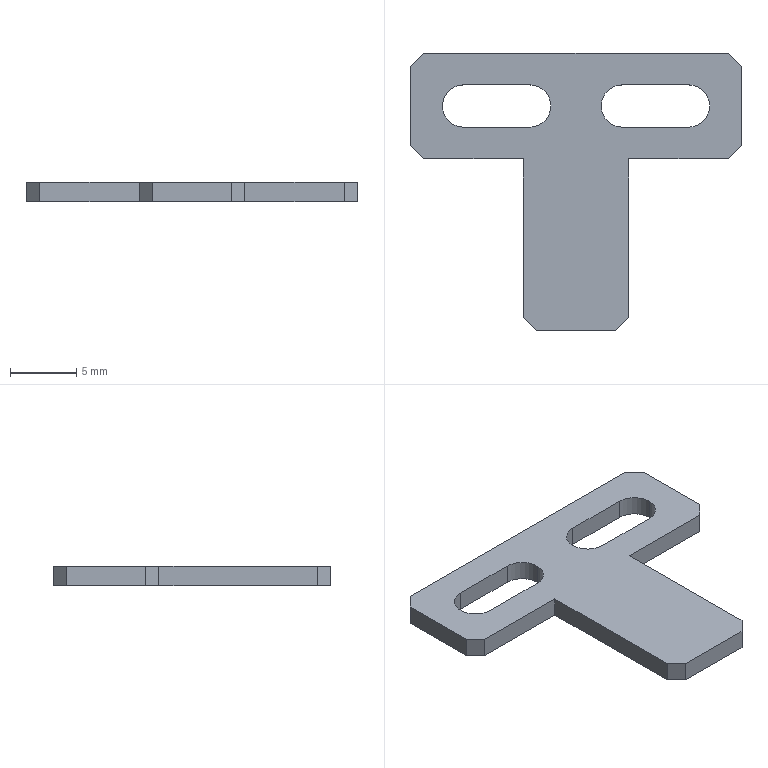Part | SolidWorks | features ICE 2, Chamfer 1, FlatPattern 1, SMBaseFlange 1, SheetMetal 1 | 1 solid | 26 faces | box 25 x 21 x 1.5 mm | volume 379.373 mm3 | plane 20 | cylinder 6 | commonest cylinder face diameters 3.2 x6
STEP:
#1=CARTESIAN_POINT('',(10.1,6.5,-1.5));
#2=VERTEX_POINT('',#1);
#3=CARTESIAN_POINT('',(8.5,8.1,-1.5));
#4=VERTEX_POINT('',#3);
#5=CARTESIAN_POINT('',(8.5,6.5,-1.5));
#6=DIRECTION('',(0.,0.,1.));
#7=DIRECTION('',(1.,0.,0.));
#8=AXIS2_PLACEMENT_3D('',#5,#6,#7);
#9=CIRCLE('',#8,1.6);
#10=EDGE_CURVE('',#2,#4,#9,.T.);
#11=ORIENTED_EDGE('',*,*,#10,.F.);
#12=CARTESIAN_POINT('',(10.1,6.5,0.));
#13=VERTEX_POINT('',#12);
#14=CARTESIAN_POINT('',(10.1,6.5,-1.5));
#15=DIRECTION('',(0.,0.,1.));
#16=VECTOR('',#15,1000.);
#17=LINE('',#14,#16);
#18=EDGE_CURVE('',#2,#13,#17,.T.);
#19=ORIENTED_EDGE('',*,*,#18,.T.);
#20=CARTESIAN_POINT('',(8.5,8.1,0.));
#21=VERTEX_POINT('',#20);
#22=CARTESIAN_POINT('',(8.5,6.5,0.));
#23=DIRECTION('',(0.,0.,1.));
#24=DIRECTION('',(1.,0.,0.));
#25=AXIS2_PLACEMENT_3D('',#22,#23,#24);
#26=CIRCLE('',#25,1.6);
#27=EDGE_CURVE('',#13,#21,#26,.T.);
#28=ORIENTED_EDGE('',*,*,#27,.T.);
#29=CARTESIAN_POINT('',(8.5,8.1,-1.5));
#30=DIRECTION('',(0.,0.,1.));
#31=VECTOR('',#30,1000.);
#32=LINE('',#29,#31);
#33=EDGE_CURVE('',#4,#21,#32,.T.);
#34=ORIENTED_EDGE('',*,*,#33,.F.);
#35=EDGE_LOOP('',(#11,#19,#28,#34));
#36=FACE_OUTER_BOUND('',#35,.T.);
#37=CARTESIAN_POINT('',(8.5,6.5,-1.5));
#38=DIRECTION('',(0.,0.,1.));
#39=DIRECTION('',(1.,0.,0.));
#40=AXIS2_PLACEMENT_3D('',#37,#38,#39);
#41=CYLINDRICAL_SURFACE('',#40,1.6);
#42=ADVANCED_FACE('',(#36),#41,.F.);
#43=CARTESIAN_POINT('',(-1.9,6.5,-1.5));
#44=VERTEX_POINT('',#43);
#45=CARTESIAN_POINT('',(-3.5,8.1,-1.5));
#46=VERTEX_POINT('',#45);
#47=CARTESIAN_POINT('',(-3.5,6.5,-1.5));
#48=DIRECTION('',(0.,0.,1.));
#49=DIRECTION('',(1.,0.,0.));
#50=AXIS2_PLACEMENT_3D('',#47,#48,#49);
#51=CIRCLE('',#50,1.6);
#52=EDGE_CURVE('',#44,#46,#51,.T.);
#53=ORIENTED_EDGE('',*,*,#52,.F.);
#54=CARTESIAN_POINT('',(-1.9,6.5,0.));
#55=VERTEX_POINT('',#54);
#56=CARTESIAN_POINT('',(-1.9,6.5,-1.5));
#57=DIRECTION('',(0.,0.,1.));
#58=VECTOR('',#57,1000.);
#59=LINE('',#56,#58);
#60=EDGE_CURVE('',#44,#55,#59,.T.);
#61=ORIENTED_EDGE('',*,*,#60,.T.);
#62=CARTESIAN_POINT('',(-3.5,8.1,0.));
#63=VERTEX_POINT('',#62);
#64=CARTESIAN_POINT('',(-3.5,6.5,0.));
#65=DIRECTION('',(0.,0.,1.));
#66=DIRECTION('',(1.,0.,0.));
#67=AXIS2_PLACEMENT_3D('',#64,#65,#66);
#68=CIRCLE('',#67,1.6);
#69=EDGE_CURVE('',#55,#63,#68,.T.);
#70=ORIENTED_EDGE('',*,*,#69,.T.);
#71=CARTESIAN_POINT('',(-3.5,8.1,-1.5));
#72=DIRECTION('',(0.,0.,1.));
#73=VECTOR('',#72,1000.);
#74=LINE('',#71,#73);
#75=EDGE_CURVE('',#46,#63,#74,.T.);
#76=ORIENTED_EDGE('',*,*,#75,.F.);
#77=EDGE_LOOP('',(#53,#61,#70,#76));
#78=FACE_OUTER_BOUND('',#77,.T.);
#79=CARTESIAN_POINT('',(-3.5,6.5,-1.5));
#80=DIRECTION('',(0.,0.,1.));
#81=DIRECTION('',(1.,0.,0.));
#82=AXIS2_PLACEMENT_3D('',#79,#80,#81);
#83=CYLINDRICAL_SURFACE('',#82,1.6);
#84=ADVANCED_FACE('',(#78),#83,.F.);
#85=CARTESIAN_POINT('',(12.5,3.5,0.));
#86=VERTEX_POINT('',#85);
#87=CARTESIAN_POINT('',(12.5,9.5,0.));
#88=VERTEX_POINT('',#87);
#89=CARTESIAN_POINT('',(12.5,10.5,0.));
#90=DIRECTION('',(0.,1.,0.));
#91=VECTOR('',#90,1000.);
#92=LINE('',#89,#91);
#93=EDGE_CURVE('',#86,#88,#92,.T.);
#94=ORIENTED_EDGE('',*,*,#93,.F.);
#95=CARTESIAN_POINT('',(12.5,3.5,-1.5));
#96=VERTEX_POINT('',#95);
#97=CARTESIAN_POINT('',(12.5,3.5,-1.5));
#98=DIRECTION('',(0.,0.,-1.));
#99=VECTOR('',#98,1000.);
#100=LINE('',#97,#99);
#101=EDGE_CURVE('',#86,#96,#100,.T.);
#102=ORIENTED_EDGE('',*,*,#101,.T.);
#103=CARTESIAN_POINT('',(12.5,9.5,-1.5));
#104=VERTEX_POINT('',#103);
#105=CARTESIAN_POINT('',(12.5,10.5,-1.5));
#106=DIRECTION('',(0.,1.,0.));
#107=VECTOR('',#106,1000.);
#108=LINE('',#105,#107);
#109=EDGE_CURVE('',#96,#104,#108,.T.);
#110=ORIENTED_EDGE('',*,*,#109,.T.);
#111=CARTESIAN_POINT('',(12.5,9.5,-1.5));
#112=DIRECTION('',(0.,0.,1.));
#113=VECTOR('',#112,1000.);
#114=LINE('',#111,#113);
#115=EDGE_CURVE('',#104,#88,#114,.T.);
#116=ORIENTED_EDGE('',*,*,#115,.T.);
#117=EDGE_LOOP('',(#94,#102,#110,#116));
#118=FACE_OUTER_BOUND('',#117,.T.);
#119=CARTESIAN_POINT('',(12.5,10.5,-1.5));
#120=DIRECTION('',(1.,0.,0.));
#121=DIRECTION('',(0.,1.,0.));
#122=AXIS2_PLACEMENT_3D('',#119,#120,#121);
#123=PLANE('',#122);
#124=ADVANCED_FACE('',(#118),#123,.T.);
#125=CARTESIAN_POINT('',(-3.,-10.5,0.));
#126=VERTEX_POINT('',#125);
#127=CARTESIAN_POINT('',(3.,-10.5,0.));
#128=VERTEX_POINT('',#127);
#129=CARTESIAN_POINT('',(-12.5,-10.5,0.));
#130=DIRECTION('',(1.,0.,0.));
#131=VECTOR('',#130,1000.);
#132=LINE('',#129,#131);
#133=EDGE_CURVE('',#126,#128,#132,.T.);
#134=ORIENTED_EDGE('',*,*,#133,.F.);
#135=CARTESIAN_POINT('',(-3.,-10.5,-1.5));
#136=VERTEX_POINT('',#135);
#137=CARTESIAN_POINT('',(-3.,-10.5,-1.5));
#138=DIRECTION('',(0.,0.,-1.));
#139=VECTOR('',#138,1000.);
#140=LINE('',#137,#139);
#141=EDGE_CURVE('',#126,#136,#140,.T.);
#142=ORIENTED_EDGE('',*,*,#141,.T.);
#143=CARTESIAN_POINT('',(3.,-10.5,-1.5));
#144=VERTEX_POINT('',#143);
#145=CARTESIAN_POINT('',(-12.5,-10.5,-1.5));
#146=DIRECTION('',(1.,0.,0.));
#147=VECTOR('',#146,1000.);
#148=LINE('',#145,#147);
#149=EDGE_CURVE('',#136,#144,#148,.T.);
#150=ORIENTED_EDGE('',*,*,#149,.T.);
#151=CARTESIAN_POINT('',(3.,-10.5,0.));
#152=DIRECTION('',(0.,0.,1.));
#153=VECTOR('',#152,1000.);
#154=LINE('',#151,#153);
#155=EDGE_CURVE('',#144,#128,#154,.T.);
#156=ORIENTED_EDGE('',*,*,#155,.T.);
#157=EDGE_LOOP('',(#134,#142,#150,#156));
#158=FACE_OUTER_BOUND('',#157,.T.);
#159=CARTESIAN_POINT('',(-12.5,-10.5,-1.5));
#160=DIRECTION('',(0.,-1.,0.));
#161=DIRECTION('',(0.,0.,-1.));
#162=AXIS2_PLACEMENT_3D('',#159,#160,#161);
#163=PLANE('',#162);
#164=ADVANCED_FACE('',(#158),#163,.T.);
#165=CARTESIAN_POINT('',(-12.5,9.5,-1.5));
#166=VERTEX_POINT('',#165);
#167=CARTESIAN_POINT('',(-12.5,3.5,-1.5));
#168=VERTEX_POINT('',#167);
#169=CARTESIAN_POINT('',(-12.5,10.5,-1.5));
#170=DIRECTION('',(0.,-1.,0.));
#171=VECTOR('',#170,1000.);
#172=LINE('',#169,#171);
#173=EDGE_CURVE('',#166,#168,#172,.T.);
#174=ORIENTED_EDGE('',*,*,#173,.T.);
#175=CARTESIAN_POINT('',(-12.5,3.5,0.));
#176=VERTEX_POINT('',#175);
#177=CARTESIAN_POINT('',(-12.5,3.5,0.));
#178=DIRECTION('',(0.,0.,1.));
#179=VECTOR('',#178,1000.);
#180=LINE('',#177,#179);
#181=EDGE_CURVE('',#168,#176,#180,.T.);
#182=ORIENTED_EDGE('',*,*,#181,.T.);
#183=CARTESIAN_POINT('',(-12.5,9.5,0.));
#184=VERTEX_POINT('',#183);
#185=CARTESIAN_POINT('',(-12.5,10.5,0.));
#186=DIRECTION('',(0.,-1.,0.));
#187=VECTOR('',#186,1000.);
#188=LINE('',#185,#187);
#189=EDGE_CURVE('',#184,#176,#188,.T.);
#190=ORIENTED_EDGE('',*,*,#189,.F.);
#191=CARTESIAN_POINT('',(-12.5,9.5,-1.5));
#192=DIRECTION('',(0.,0.,-1.));
#193=VECTOR('',#192,1000.);
#194=LINE('',#191,#193);
#195=EDGE_CURVE('',#184,#166,#194,.T.);
#196=ORIENTED_EDGE('',*,*,#195,.T.);
#197=EDGE_LOOP('',(#174,#182,#190,#196));
#198=FACE_OUTER_BOUND('',#197,.T.);
#199=CARTESIAN_POINT('',(-12.5,10.5,-1.5));
#200=DIRECTION('',(-1.,0.,0.));
#201=DIRECTION('',(0.,-1.,0.));
#202=AXIS2_PLACEMENT_3D('',#199,#200,#201);
#203=PLANE('',#202);
#204=ADVANCED_FACE('',(#198),#203,.T.);
#205=CARTESIAN_POINT('',(11.5,10.5,-1.5));
#206=VERTEX_POINT('',#205);
#207=CARTESIAN_POINT('',(-11.5,10.5,-1.5));
#208=VERTEX_POINT('',#207);
#209=CARTESIAN_POINT('',(-12.5,10.5,-1.5));
#210=DIRECTION('',(-1.,0.,0.));
#211=VECTOR('',#210,1000.);
#212=LINE('',#209,#211);
#213=EDGE_CURVE('',#206,#208,#212,.T.);
#214=ORIENTED_EDGE('',*,*,#213,.T.);
#215=CARTESIAN_POINT('',(-11.5,10.5,0.));
#216=VERTEX_POINT('',#215);
#217=CARTESIAN_POINT('',(-11.5,10.5,-1.5));
#218=DIRECTION('',(0.,0.,1.));
#219=VECTOR('',#218,1000.);
#220=LINE('',#217,#219);
#221=EDGE_CURVE('',#208,#216,#220,.T.);
#222=ORIENTED_EDGE('',*,*,#221,.T.);
#223=CARTESIAN_POINT('',(11.5,10.5,0.));
#224=VERTEX_POINT('',#223);
#225=CARTESIAN_POINT('',(-12.5,10.5,0.));
#226=DIRECTION('',(-1.,0.,0.));
#227=VECTOR('',#226,1000.);
#228=LINE('',#225,#227);
#229=EDGE_CURVE('',#224,#216,#228,.T.);
#230=ORIENTED_EDGE('',*,*,#229,.F.);
#231=CARTESIAN_POINT('',(11.5,10.5,-1.5));
#232=DIRECTION('',(0.,0.,-1.));
#233=VECTOR('',#232,1000.);
#234=LINE('',#231,#233);
#235=EDGE_CURVE('',#224,#206,#234,.T.);
#236=ORIENTED_EDGE('',*,*,#235,.T.);
#237=EDGE_LOOP('',(#214,#222,#230,#236));
#238=FACE_OUTER_BOUND('',#237,.T.);
#239=CARTESIAN_POINT('',(-12.5,10.5,-1.5));
#240=DIRECTION('',(0.,1.,0.));
#241=DIRECTION('',(0.,0.,1.));
#242=AXIS2_PLACEMENT_3D('',#239,#240,#241);
#243=PLANE('',#242);
#244=ADVANCED_FACE('',(#238),#243,.T.);
#245=CARTESIAN_POINT('',(3.5,8.1,-1.5));
#246=VERTEX_POINT('',#245);
#247=CARTESIAN_POINT('',(3.5,8.1,-1.5));
#248=DIRECTION('',(-1.,0.,0.));
#249=VECTOR('',#248,1000.);
#250=LINE('',#247,#249);
#251=EDGE_CURVE('',#4,#246,#250,.T.);
#252=ORIENTED_EDGE('',*,*,#251,.T.);
#253=CARTESIAN_POINT('',(3.5,4.9,-1.5));
#254=VERTEX_POINT('',#253);
#255=CARTESIAN_POINT('',(3.5,6.5,-1.5));
#256=DIRECTION('',(0.,0.,1.));
#257=DIRECTION('',(1.,0.,0.));
#258=AXIS2_PLACEMENT_3D('',#255,#256,#257);
#259=CIRCLE('',#258,1.6);
#260=EDGE_CURVE('',#246,#254,#259,.T.);
#261=ORIENTED_EDGE('',*,*,#260,.T.);
#262=CARTESIAN_POINT('',(8.5,4.9,-1.5));
#263=VERTEX_POINT('',#262);
#264=CARTESIAN_POINT('',(3.5,4.9,-1.5));
#265=DIRECTION('',(1.,0.,0.));
#266=VECTOR('',#265,1000.);
#267=LINE('',#264,#266);
#268=EDGE_CURVE('',#254,#263,#267,.T.);
#269=ORIENTED_EDGE('',*,*,#268,.T.);
#270=CARTESIAN_POINT('',(8.5,6.5,-1.5));
#271=DIRECTION('',(0.,0.,1.));
#272=DIRECTION('',(1.,0.,0.));
#273=AXIS2_PLACEMENT_3D('',#270,#271,#272);
#274=CIRCLE('',#273,1.6);
#275=EDGE_CURVE('',#263,#2,#274,.T.);
#276=ORIENTED_EDGE('',*,*,#275,.T.);
#277=ORIENTED_EDGE('',*,*,#10,.T.);
#278=EDGE_LOOP('',(#252,#261,#269,#276,#277));
#279=FACE_BOUND('',#278,.T.);
#280=CARTESIAN_POINT('',(-8.5,8.1,-1.5));
#281=VERTEX_POINT('',#280);
#282=CARTESIAN_POINT('',(-8.5,8.1,-1.5));
#283=DIRECTION('',(-1.,0.,0.));
#284=VECTOR('',#283,1000.);
#285=LINE('',#282,#284);
#286=EDGE_CURVE('',#46,#281,#285,.T.);
#287=ORIENTED_EDGE('',*,*,#286,.T.);
#288=CARTESIAN_POINT('',(-8.5,4.9,-1.5));
#289=VERTEX_POINT('',#288);
#290=CARTESIAN_POINT('',(-8.5,6.5,-1.5));
#291=DIRECTION('',(0.,0.,1.));
#292=DIRECTION('',(1.,0.,0.));
#293=AXIS2_PLACEMENT_3D('',#290,#291,#292);
#294=CIRCLE('',#293,1.6);
#295=EDGE_CURVE('',#281,#289,#294,.T.);
#296=ORIENTED_EDGE('',*,*,#295,.T.);
#297=CARTESIAN_POINT('',(-3.5,4.9,-1.5));
#298=VERTEX_POINT('',#297);
#299=CARTESIAN_POINT('',(-8.5,4.9,-1.5));
#300=DIRECTION('',(1.,0.,0.));
#301=VECTOR('',#300,1000.);
#302=LINE('',#299,#301);
#303=EDGE_CURVE('',#289,#298,#302,.T.);
#304=ORIENTED_EDGE('',*,*,#303,.T.);
#305=CARTESIAN_POINT('',(-3.5,6.5,-1.5));
#306=DIRECTION('',(0.,0.,1.));
#307=DIRECTION('',(1.,0.,0.));
#308=AXIS2_PLACEMENT_3D('',#305,#306,#307);
#309=CIRCLE('',#308,1.6);
#310=EDGE_CURVE('',#298,#44,#309,.T.);
#311=ORIENTED_EDGE('',*,*,#310,.T.);
#312=ORIENTED_EDGE('',*,*,#52,.T.);
#313=EDGE_LOOP('',(#287,#296,#304,#311,#312));
#314=FACE_BOUND('',#313,.T.);
#315=ORIENTED_EDGE('',*,*,#149,.F.);
#316=CARTESIAN_POINT('',(-4.,-9.5,-1.5));
#317=VERTEX_POINT('',#316);
#318=CARTESIAN_POINT('',(-4.,-9.5,-1.5));
#319=DIRECTION('',(-0.7071,0.7071,0.));
#320=VECTOR('',#319,1000.);
#321=LINE('',#318,#320);
#322=EDGE_CURVE('',#136,#317,#321,.T.);
#323=ORIENTED_EDGE('',*,*,#322,.T.);
#324=CARTESIAN_POINT('',(-4.,2.5,-1.5));
#325=VERTEX_POINT('',#324);
#326=CARTESIAN_POINT('',(-4.,-10.5,-1.5));
#327=DIRECTION('',(0.,1.,0.));
#328=VECTOR('',#327,1000.);
#329=LINE('',#326,#328);
#330=EDGE_CURVE('',#317,#325,#329,.T.);
#331=ORIENTED_EDGE('',*,*,#330,.T.);
#332=CARTESIAN_POINT('',(-11.5,2.5,-1.5));
#333=VERTEX_POINT('',#332);
#334=CARTESIAN_POINT('',(-12.5,2.5,-1.5));
#335=DIRECTION('',(-1.,0.,0.));
#336=VECTOR('',#335,1000.);
#337=LINE('',#334,#336);
#338=EDGE_CURVE('',#325,#333,#337,.T.);
#339=ORIENTED_EDGE('',*,*,#338,.T.);
#340=CARTESIAN_POINT('',(-12.5,3.5,-1.5));
#341=DIRECTION('',(-0.7071,0.7071,0.));
#342=VECTOR('',#341,1000.);
#343=LINE('',#340,#342);
#344=EDGE_CURVE('',#333,#168,#343,.T.);
#345=ORIENTED_EDGE('',*,*,#344,.T.);
#346=ORIENTED_EDGE('',*,*,#173,.F.);
#347=CARTESIAN_POINT('',(-11.5,10.5,-1.5));
#348=DIRECTION('',(0.7071,0.7071,0.));
#349=VECTOR('',#348,1000.);
#350=LINE('',#347,#349);
#351=EDGE_CURVE('',#166,#208,#350,.T.);
#352=ORIENTED_EDGE('',*,*,#351,.T.);
#353=ORIENTED_EDGE('',*,*,#213,.F.);
#354=CARTESIAN_POINT('',(12.5,9.5,-1.5));
#355=DIRECTION('',(0.7071,-0.7071,0.));
#356=VECTOR('',#355,1000.);
#357=LINE('',#354,#356);
#358=EDGE_CURVE('',#206,#104,#357,.T.);
#359=ORIENTED_EDGE('',*,*,#358,.T.);
#360=ORIENTED_EDGE('',*,*,#109,.F.);
#361=CARTESIAN_POINT('',(11.5,2.5,-1.5));
#362=VERTEX_POINT('',#361);
#363=CARTESIAN_POINT('',(11.5,2.5,-1.5));
#364=DIRECTION('',(-0.7071,-0.7071,0.));
#365=VECTOR('',#364,1000.);
#366=LINE('',#363,#365);
#367=EDGE_CURVE('',#96,#362,#366,.T.);
#368=ORIENTED_EDGE('',*,*,#367,.T.);
#369=CARTESIAN_POINT('',(4.,2.5,-1.5));
#370=VERTEX_POINT('',#369);
#371=CARTESIAN_POINT('',(12.5,2.5,-1.5));
#372=DIRECTION('',(-1.,0.,0.));
#373=VECTOR('',#372,1000.);
#374=LINE('',#371,#373);
#375=EDGE_CURVE('',#362,#370,#374,.T.);
#376=ORIENTED_EDGE('',*,*,#375,.T.);
#377=CARTESIAN_POINT('',(4.,-9.5,-1.5));
#378=VERTEX_POINT('',#377);
#379=CARTESIAN_POINT('',(4.,-10.5,-1.5));
#380=DIRECTION('',(0.,-1.,0.));
#381=VECTOR('',#380,1000.);
#382=LINE('',#379,#381);
#383=EDGE_CURVE('',#370,#378,#382,.T.);
#384=ORIENTED_EDGE('',*,*,#383,.T.);
#385=CARTESIAN_POINT('',(3.,-10.5,-1.5));
#386=DIRECTION('',(-0.7071,-0.7071,0.));
#387=VECTOR('',#386,1000.);
#388=LINE('',#385,#387);
#389=EDGE_CURVE('',#378,#144,#388,.T.);
#390=ORIENTED_EDGE('',*,*,#389,.T.);
#391=EDGE_LOOP('',(#315,#323,#331,#339,#345,#346,#352,#353,#359,#360,#368,#376,#384,#390));
#392=FACE_OUTER_BOUND('',#391,.T.);
#393=CARTESIAN_POINT('',(0.,0.,-1.5));
#394=DIRECTION('',(0.,0.,1.));
#395=DIRECTION('',(1.,0.,0.));
#396=AXIS2_PLACEMENT_3D('',#393,#394,#395);
#397=PLANE('',#396);
#398=ADVANCED_FACE('',(#279,#314,#392),#397,.F.);
#399=CARTESIAN_POINT('',(-4.,-9.5,0.));
#400=VERTEX_POINT('',#399);
#401=CARTESIAN_POINT('',(-4.,2.5,0.));
#402=VERTEX_POINT('',#401);
#403=CARTESIAN_POINT('',(-4.,-10.5,0.));
#404=DIRECTION('',(0.,1.,0.));
#405=VECTOR('',#404,1000.);
#406=LINE('',#403,#405);
#407=EDGE_CURVE('',#400,#402,#406,.T.);
#408=ORIENTED_EDGE('',*,*,#407,.F.);
#409=CARTESIAN_POINT('',(-6.75,-6.75,0.));
#410=DIRECTION('',(0.7071,-0.7071,0.));
#411=VECTOR('',#410,1000.);
#412=LINE('',#409,#411);
#413=EDGE_CURVE('',#400,#126,#412,.T.);
#414=ORIENTED_EDGE('',*,*,#413,.T.);
#415=ORIENTED_EDGE('',*,*,#133,.T.);
#416=CARTESIAN_POINT('',(4.,-9.5,0.));
#417=VERTEX_POINT('',#416);
#418=CARTESIAN_POINT('',(6.75,-6.75,0.));
#419=DIRECTION('',(0.7071,0.7071,0.));
#420=VECTOR('',#419,1000.);
#421=LINE('',#418,#420);
#422=EDGE_CURVE('',#128,#417,#421,.T.);
#423=ORIENTED_EDGE('',*,*,#422,.T.);
#424=CARTESIAN_POINT('',(4.,2.5,0.));
#425=VERTEX_POINT('',#424);
#426=CARTESIAN_POINT('',(4.,-10.5,0.));
#427=DIRECTION('',(0.,-1.,0.));
#428=VECTOR('',#427,1000.);
#429=LINE('',#426,#428);
#430=EDGE_CURVE('',#425,#417,#429,.T.);
#431=ORIENTED_EDGE('',*,*,#430,.F.);
#432=CARTESIAN_POINT('',(11.5,2.5,0.));
#433=VERTEX_POINT('',#432);
#434=CARTESIAN_POINT('',(12.5,2.5,0.));
#435=DIRECTION('',(-1.,0.,0.));
#436=VECTOR('',#435,1000.);
#437=LINE('',#434,#436);
#438=EDGE_CURVE('',#433,#425,#437,.T.);
#439=ORIENTED_EDGE('',*,*,#438,.F.);
#440=CARTESIAN_POINT('',(4.5,-4.5,0.));
#441=DIRECTION('',(0.7071,0.7071,0.));
#442=VECTOR('',#441,1000.);
#443=LINE('',#440,#442);
#444=EDGE_CURVE('',#433,#86,#443,.T.);
#445=ORIENTED_EDGE('',*,*,#444,.T.);
#446=ORIENTED_EDGE('',*,*,#93,.T.);
#447=CARTESIAN_POINT('',(11.,11.,0.));
#448=DIRECTION('',(-0.7071,0.7071,0.));
#449=VECTOR('',#448,1000.);
#450=LINE('',#447,#449);
#451=EDGE_CURVE('',#88,#224,#450,.T.);
#452=ORIENTED_EDGE('',*,*,#451,.T.);
#453=ORIENTED_EDGE('',*,*,#229,.T.);
#454=CARTESIAN_POINT('',(-11.,11.,0.));
#455=DIRECTION('',(-0.7071,-0.7071,0.));
#456=VECTOR('',#455,1000.);
#457=LINE('',#454,#456);
#458=EDGE_CURVE('',#216,#184,#457,.T.);
#459=ORIENTED_EDGE('',*,*,#458,.T.);
#460=ORIENTED_EDGE('',*,*,#189,.T.);
#461=CARTESIAN_POINT('',(-11.5,2.5,0.));
#462=VERTEX_POINT('',#461);
#463=CARTESIAN_POINT('',(-4.5,-4.5,0.));
#464=DIRECTION('',(0.7071,-0.7071,0.));
#465=VECTOR('',#464,1000.);
#466=LINE('',#463,#465);
#467=EDGE_CURVE('',#176,#462,#466,.T.);
#468=ORIENTED_EDGE('',*,*,#467,.T.);
#469=CARTESIAN_POINT('',(-12.5,2.5,0.));
#470=DIRECTION('',(-1.,0.,0.));
#471=VECTOR('',#470,1000.);
#472=LINE('',#469,#471);
#473=EDGE_CURVE('',#402,#462,#472,.T.);
#474=ORIENTED_EDGE('',*,*,#473,.F.);
#475=EDGE_LOOP('',(#408,#414,#415,#423,#431,#439,#445,#446,#452,#453,#459,#460,#468,#474));
#476=FACE_OUTER_BOUND('',#475,.T.);
#477=CARTESIAN_POINT('',(3.5,8.1,0.));
#478=VERTEX_POINT('',#477);
#479=CARTESIAN_POINT('',(3.5,4.9,0.));
#480=VERTEX_POINT('',#479);
#481=CARTESIAN_POINT('',(3.5,6.5,0.));
#482=DIRECTION('',(0.,0.,1.));
#483=DIRECTION('',(1.,0.,0.));
#484=AXIS2_PLACEMENT_3D('',#481,#482,#483);
#485=CIRCLE('',#484,1.6);
#486=EDGE_CURVE('',#478,#480,#485,.T.);
#487=ORIENTED_EDGE('',*,*,#486,.F.);
#488=CARTESIAN_POINT('',(3.5,8.1,0.));
#489=DIRECTION('',(-1.,0.,0.));
#490=VECTOR('',#489,1000.);
#491=LINE('',#488,#490);
#492=EDGE_CURVE('',#21,#478,#491,.T.);
#493=ORIENTED_EDGE('',*,*,#492,.F.);
#494=ORIENTED_EDGE('',*,*,#27,.F.);
#495=CARTESIAN_POINT('',(8.5,4.9,0.));
#496=VERTEX_POINT('',#495);
#497=CARTESIAN_POINT('',(8.5,6.5,0.));
#498=DIRECTION('',(0.,0.,1.));
#499=DIRECTION('',(1.,0.,0.));
#500=AXIS2_PLACEMENT_3D('',#497,#498,#499);
#501=CIRCLE('',#500,1.6);
#502=EDGE_CURVE('',#496,#13,#501,.T.);
#503=ORIENTED_EDGE('',*,*,#502,.F.);
#504=CARTESIAN_POINT('',(3.5,4.9,0.));
#505=DIRECTION('',(1.,0.,0.));
#506=VECTOR('',#505,1000.);
#507=LINE('',#504,#506);
#508=EDGE_CURVE('',#480,#496,#507,.T.);
#509=ORIENTED_EDGE('',*,*,#508,.F.);
#510=EDGE_LOOP('',(#487,#493,#494,#503,#509));
#511=FACE_BOUND('',#510,.T.);
#512=CARTESIAN_POINT('',(-8.5,8.1,0.));
#513=VERTEX_POINT('',#512);
#514=CARTESIAN_POINT('',(-8.5,4.9,0.));
#515=VERTEX_POINT('',#514);
#516=CARTESIAN_POINT('',(-8.5,6.5,0.));
#517=DIRECTION('',(0.,0.,1.));
#518=DIRECTION('',(1.,0.,0.));
#519=AXIS2_PLACEMENT_3D('',#516,#517,#518);
#520=CIRCLE('',#519,1.6);
#521=EDGE_CURVE('',#513,#515,#520,.T.);
#522=ORIENTED_EDGE('',*,*,#521,.F.);
#523=CARTESIAN_POINT('',(-8.5,8.1,0.));
#524=DIRECTION('',(-1.,0.,0.));
#525=VECTOR('',#524,1000.);
#526=LINE('',#523,#525);
#527=EDGE_CURVE('',#63,#513,#526,.T.);
#528=ORIENTED_EDGE('',*,*,#527,.F.);
#529=ORIENTED_EDGE('',*,*,#69,.F.);
#530=CARTESIAN_POINT('',(-3.5,4.9,0.));
#531=VERTEX_POINT('',#530);
#532=CARTESIAN_POINT('',(-3.5,6.5,0.));
#533=DIRECTION('',(0.,0.,1.));
#534=DIRECTION('',(1.,0.,0.));
#535=AXIS2_PLACEMENT_3D('',#532,#533,#534);
#536=CIRCLE('',#535,1.6);
#537=EDGE_CURVE('',#531,#55,#536,.T.);
#538=ORIENTED_EDGE('',*,*,#537,.F.);
#539=CARTESIAN_POINT('',(-8.5,4.9,0.));
#540=DIRECTION('',(1.,0.,0.));
#541=VECTOR('',#540,1000.);
#542=LINE('',#539,#541);
#543=EDGE_CURVE('',#515,#531,#542,.T.);
#544=ORIENTED_EDGE('',*,*,#543,.F.);
#545=EDGE_LOOP('',(#522,#528,#529,#538,#544));
#546=FACE_BOUND('',#545,.T.);
#547=CARTESIAN_POINT('',(0.,0.,0.));
#548=DIRECTION('',(0.,0.,1.));
#549=DIRECTION('',(1.,0.,0.));
#550=AXIS2_PLACEMENT_3D('',#547,#548,#549);
#551=PLANE('',#550);
#552=ADVANCED_FACE('',(#476,#511,#546),#551,.T.);
#553=ORIENTED_EDGE('',*,*,#521,.T.);
#554=CARTESIAN_POINT('',(-8.5,4.9,-1.5));
#555=DIRECTION('',(0.,0.,1.));
#556=VECTOR('',#555,1000.);
#557=LINE('',#554,#556);
#558=EDGE_CURVE('',#289,#515,#557,.T.);
#559=ORIENTED_EDGE('',*,*,#558,.F.);
#560=ORIENTED_EDGE('',*,*,#295,.F.);
#561=CARTESIAN_POINT('',(-8.5,8.1,-1.5));
#562=DIRECTION('',(0.,0.,1.));
#563=VECTOR('',#562,1000.);
#564=LINE('',#561,#563);
#565=EDGE_CURVE('',#281,#513,#564,.T.);
#566=ORIENTED_EDGE('',*,*,#565,.T.);
#567=EDGE_LOOP('',(#553,#559,#560,#566));
#568=FACE_OUTER_BOUND('',#567,.T.);
#569=CARTESIAN_POINT('',(-8.5,6.5,-1.5));
#570=DIRECTION('',(0.,0.,1.));
#571=DIRECTION('',(1.,0.,0.));
#572=AXIS2_PLACEMENT_3D('',#569,#570,#571);
#573=CYLINDRICAL_SURFACE('',#572,1.6);
#574=ADVANCED_FACE('',(#568),#573,.F.);
#575=ORIENTED_EDGE('',*,*,#527,.T.);
#576=ORIENTED_EDGE('',*,*,#565,.F.);
#577=ORIENTED_EDGE('',*,*,#286,.F.);
#578=ORIENTED_EDGE('',*,*,#75,.T.);
#579=EDGE_LOOP('',(#575,#576,#577,#578));
#580=FACE_OUTER_BOUND('',#579,.T.);
#581=CARTESIAN_POINT('',(-8.5,8.1,-1.5));
#582=DIRECTION('',(0.,1.,0.));
#583=DIRECTION('',(-1.,0.,0.));
#584=AXIS2_PLACEMENT_3D('',#581,#582,#583);
#585=PLANE('',#584);
#586=ADVANCED_FACE('',(#580),#585,.F.);
#587=ORIENTED_EDGE('',*,*,#60,.F.);
#588=ORIENTED_EDGE('',*,*,#310,.F.);
#589=CARTESIAN_POINT('',(-3.5,4.9,-1.5));
#590=DIRECTION('',(0.,0.,1.));
#591=VECTOR('',#590,1000.);
#592=LINE('',#589,#591);
#593=EDGE_CURVE('',#298,#531,#592,.T.);
#594=ORIENTED_EDGE('',*,*,#593,.T.);
#595=ORIENTED_EDGE('',*,*,#537,.T.);
#596=EDGE_LOOP('',(#587,#588,#594,#595));
#597=FACE_OUTER_BOUND('',#596,.T.);
#598=CARTESIAN_POINT('',(-3.5,6.5,-1.5));
#599=DIRECTION('',(0.,0.,1.));
#600=DIRECTION('',(1.,0.,0.));
#601=AXIS2_PLACEMENT_3D('',#598,#599,#600);
#602=CYLINDRICAL_SURFACE('',#601,1.6);
#603=ADVANCED_FACE('',(#597),#602,.F.);
#604=ORIENTED_EDGE('',*,*,#543,.T.);
#605=ORIENTED_EDGE('',*,*,#593,.F.);
#606=ORIENTED_EDGE('',*,*,#303,.F.);
#607=ORIENTED_EDGE('',*,*,#558,.T.);
#608=EDGE_LOOP('',(#604,#605,#606,#607));
#609=FACE_OUTER_BOUND('',#608,.T.);
#610=CARTESIAN_POINT('',(-8.5,4.9,-1.5));
#611=DIRECTION('',(0.,-1.,0.));
#612=DIRECTION('',(1.,0.,0.));
#613=AXIS2_PLACEMENT_3D('',#610,#611,#612);
#614=PLANE('',#613);
#615=ADVANCED_FACE('',(#609),#614,.F.);
#616=ORIENTED_EDGE('',*,*,#486,.T.);
#617=CARTESIAN_POINT('',(3.5,4.9,-1.5));
#618=DIRECTION('',(0.,0.,1.));
#619=VECTOR('',#618,1000.);
#620=LINE('',#617,#619);
#621=EDGE_CURVE('',#254,#480,#620,.T.);
#622=ORIENTED_EDGE('',*,*,#621,.F.);
#623=ORIENTED_EDGE('',*,*,#260,.F.);
#624=CARTESIAN_POINT('',(3.5,8.1,-1.5));
#625=DIRECTION('',(0.,0.,1.));
#626=VECTOR('',#625,1000.);
#627=LINE('',#624,#626);
#628=EDGE_CURVE('',#246,#478,#627,.T.);
#629=ORIENTED_EDGE('',*,*,#628,.T.);
#630=EDGE_LOOP('',(#616,#622,#623,#629));
#631=FACE_OUTER_BOUND('',#630,.T.);
#632=CARTESIAN_POINT('',(3.5,6.5,-1.5));
#633=DIRECTION('',(0.,0.,1.));
#634=DIRECTION('',(1.,0.,0.));
#635=AXIS2_PLACEMENT_3D('',#632,#633,#634);
#636=CYLINDRICAL_SURFACE('',#635,1.6);
#637=ADVANCED_FACE('',(#631),#636,.F.);
#638=ORIENTED_EDGE('',*,*,#492,.T.);
#639=ORIENTED_EDGE('',*,*,#628,.F.);
#640=ORIENTED_EDGE('',*,*,#251,.F.);
#641=ORIENTED_EDGE('',*,*,#33,.T.);
#642=EDGE_LOOP('',(#638,#639,#640,#641));
#643=FACE_OUTER_BOUND('',#642,.T.);
#644=CARTESIAN_POINT('',(3.5,8.1,-1.5));
#645=DIRECTION('',(0.,1.,0.));
#646=DIRECTION('',(-1.,0.,0.));
#647=AXIS2_PLACEMENT_3D('',#644,#645,#646);
#648=PLANE('',#647);
#649=ADVANCED_FACE('',(#643),#648,.F.);
#650=ORIENTED_EDGE('',*,*,#18,.F.);
#651=ORIENTED_EDGE('',*,*,#275,.F.);
#652=CARTESIAN_POINT('',(8.5,4.9,-1.5));
#653=DIRECTION('',(0.,0.,1.));
#654=VECTOR('',#653,1000.);
#655=LINE('',#652,#654);
#656=EDGE_CURVE('',#263,#496,#655,.T.);
#657=ORIENTED_EDGE('',*,*,#656,.T.);
#658=ORIENTED_EDGE('',*,*,#502,.T.);
#659=EDGE_LOOP('',(#650,#651,#657,#658));
#660=FACE_OUTER_BOUND('',#659,.T.);
#661=CARTESIAN_POINT('',(8.5,6.5,-1.5));
#662=DIRECTION('',(0.,0.,1.));
#663=DIRECTION('',(1.,0.,0.));
#664=AXIS2_PLACEMENT_3D('',#661,#662,#663);
#665=CYLINDRICAL_SURFACE('',#664,1.6);
#666=ADVANCED_FACE('',(#660),#665,.F.);
#667=ORIENTED_EDGE('',*,*,#508,.T.);
#668=ORIENTED_EDGE('',*,*,#656,.F.);
#669=ORIENTED_EDGE('',*,*,#268,.F.);
#670=ORIENTED_EDGE('',*,*,#621,.T.);
#671=EDGE_LOOP('',(#667,#668,#669,#670));
#672=FACE_OUTER_BOUND('',#671,.T.);
#673=CARTESIAN_POINT('',(3.5,4.9,-1.5));
#674=DIRECTION('',(0.,-1.,0.));
#675=DIRECTION('',(1.,0.,0.));
#676=AXIS2_PLACEMENT_3D('',#673,#674,#675);
#677=PLANE('',#676);
#678=ADVANCED_FACE('',(#672),#677,.F.);
#679=ORIENTED_EDGE('',*,*,#473,.T.);
#680=CARTESIAN_POINT('',(-11.5,2.5,-1.5));
#681=DIRECTION('',(0.,0.,-1.));
#682=VECTOR('',#681,1000.);
#683=LINE('',#680,#682);
#684=EDGE_CURVE('',#462,#333,#683,.T.);
#685=ORIENTED_EDGE('',*,*,#684,.T.);
#686=ORIENTED_EDGE('',*,*,#338,.F.);
#687=CARTESIAN_POINT('',(-4.,2.5,-1.5));
#688=DIRECTION('',(0.,0.,1.));
#689=VECTOR('',#688,1000.);
#690=LINE('',#687,#689);
#691=EDGE_CURVE('',#325,#402,#690,.T.);
#692=ORIENTED_EDGE('',*,*,#691,.T.);
#693=EDGE_LOOP('',(#679,#685,#686,#692));
#694=FACE_OUTER_BOUND('',#693,.T.);
#695=CARTESIAN_POINT('',(-12.5,2.5,-1.5));
#696=DIRECTION('',(0.,1.,0.));
#697=DIRECTION('',(0.,0.,1.));
#698=AXIS2_PLACEMENT_3D('',#695,#696,#697);
#699=PLANE('',#698);
#700=ADVANCED_FACE('',(#694),#699,.F.);
#701=ORIENTED_EDGE('',*,*,#330,.F.);
#702=CARTESIAN_POINT('',(-4.,-9.5,0.));
#703=DIRECTION('',(0.,0.,1.));
#704=VECTOR('',#703,1000.);
#705=LINE('',#702,#704);
#706=EDGE_CURVE('',#317,#400,#705,.T.);
#707=ORIENTED_EDGE('',*,*,#706,.T.);
#708=ORIENTED_EDGE('',*,*,#407,.T.);
#709=ORIENTED_EDGE('',*,*,#691,.F.);
#710=EDGE_LOOP('',(#701,#707,#708,#709));
#711=FACE_OUTER_BOUND('',#710,.T.);
#712=CARTESIAN_POINT('',(-4.,-10.5,-1.5));
#713=DIRECTION('',(1.,0.,0.));
#714=DIRECTION('',(0.,1.,0.));
#715=AXIS2_PLACEMENT_3D('',#712,#713,#714);
#716=PLANE('',#715);
#717=ADVANCED_FACE('',(#711),#716,.F.);
#718=ORIENTED_EDGE('',*,*,#430,.T.);
#719=CARTESIAN_POINT('',(4.,-9.5,-1.5));
#720=DIRECTION('',(0.,0.,-1.));
#721=VECTOR('',#720,1000.);
#722=LINE('',#719,#721);
#723=EDGE_CURVE('',#417,#378,#722,.T.);
#724=ORIENTED_EDGE('',*,*,#723,.T.);
#725=ORIENTED_EDGE('',*,*,#383,.F.);
#726=CARTESIAN_POINT('',(4.,2.5,-1.5));
#727=DIRECTION('',(0.,0.,1.));
#728=VECTOR('',#727,1000.);
#729=LINE('',#726,#728);
#730=EDGE_CURVE('',#370,#425,#729,.T.);
#731=ORIENTED_EDGE('',*,*,#730,.T.);
#732=EDGE_LOOP('',(#718,#724,#725,#731));
#733=FACE_OUTER_BOUND('',#732,.T.);
#734=CARTESIAN_POINT('',(4.,-10.5,-1.5));
#735=DIRECTION('',(-1.,0.,0.));
#736=DIRECTION('',(0.,-1.,0.));
#737=AXIS2_PLACEMENT_3D('',#734,#735,#736);
#738=PLANE('',#737);
#739=ADVANCED_FACE('',(#733),#738,.F.);
#740=ORIENTED_EDGE('',*,*,#375,.F.);
#741=CARTESIAN_POINT('',(11.5,2.5,0.));
#742=DIRECTION('',(0.,0.,1.));
#743=VECTOR('',#742,1000.);
#744=LINE('',#741,#743);
#745=EDGE_CURVE('',#362,#433,#744,.T.);
#746=ORIENTED_EDGE('',*,*,#745,.T.);
#747=ORIENTED_EDGE('',*,*,#438,.T.);
#748=ORIENTED_EDGE('',*,*,#730,.F.);
#749=EDGE_LOOP('',(#740,#746,#747,#748));
#750=FACE_OUTER_BOUND('',#749,.T.);
#751=CARTESIAN_POINT('',(12.5,2.5,-1.5));
#752=DIRECTION('',(0.,1.,0.));
#753=DIRECTION('',(-1.,0.,0.));
#754=AXIS2_PLACEMENT_3D('',#751,#752,#753);
#755=PLANE('',#754);
#756=ADVANCED_FACE('',(#750),#755,.F.);
#757=ORIENTED_EDGE('',*,*,#322,.F.);
#758=ORIENTED_EDGE('',*,*,#141,.F.);
#759=ORIENTED_EDGE('',*,*,#413,.F.);
#760=ORIENTED_EDGE('',*,*,#706,.F.);
#761=EDGE_LOOP('',(#757,#758,#759,#760));
#762=FACE_OUTER_BOUND('',#761,.T.);
#763=CARTESIAN_POINT('',(-4.,-9.5,-1.5));
#764=DIRECTION('',(-0.7071,-0.7071,0.));
#765=DIRECTION('',(0.,0.,-1.));
#766=AXIS2_PLACEMENT_3D('',#763,#764,#765);
#767=PLANE('',#766);
#768=ADVANCED_FACE('',(#762),#767,.T.);
#769=ORIENTED_EDGE('',*,*,#389,.F.);
#770=ORIENTED_EDGE('',*,*,#723,.F.);
#771=ORIENTED_EDGE('',*,*,#422,.F.);
#772=ORIENTED_EDGE('',*,*,#155,.F.);
#773=EDGE_LOOP('',(#769,#770,#771,#772));
#774=FACE_OUTER_BOUND('',#773,.T.);
#775=CARTESIAN_POINT('',(3.,-10.5,-1.5));
#776=DIRECTION('',(0.7071,-0.7071,0.));
#777=DIRECTION('',(0.,0.,-1.));
#778=AXIS2_PLACEMENT_3D('',#775,#776,#777);
#779=PLANE('',#778);
#780=ADVANCED_FACE('',(#774),#779,.T.);
#781=ORIENTED_EDGE('',*,*,#344,.F.);
#782=ORIENTED_EDGE('',*,*,#684,.F.);
#783=ORIENTED_EDGE('',*,*,#467,.F.);
#784=ORIENTED_EDGE('',*,*,#181,.F.);
#785=EDGE_LOOP('',(#781,#782,#783,#784));
#786=FACE_OUTER_BOUND('',#785,.T.);
#787=CARTESIAN_POINT('',(-12.5,3.5,-1.5));
#788=DIRECTION('',(-0.7071,-0.7071,0.));
#789=DIRECTION('',(0.,0.,-1.));
#790=AXIS2_PLACEMENT_3D('',#787,#788,#789);
#791=PLANE('',#790);
#792=ADVANCED_FACE('',(#786),#791,.T.);
#793=ORIENTED_EDGE('',*,*,#351,.F.);
#794=ORIENTED_EDGE('',*,*,#195,.F.);
#795=ORIENTED_EDGE('',*,*,#458,.F.);
#796=ORIENTED_EDGE('',*,*,#221,.F.);
#797=EDGE_LOOP('',(#793,#794,#795,#796));
#798=FACE_OUTER_BOUND('',#797,.T.);
#799=CARTESIAN_POINT('',(-11.5,10.5,-1.5));
#800=DIRECTION('',(0.7071,-0.7071,0.));
#801=DIRECTION('',(0.,0.,1.));
#802=AXIS2_PLACEMENT_3D('',#799,#800,#801);
#803=PLANE('',#802);
#804=ADVANCED_FACE('',(#798),#803,.F.);
#805=ORIENTED_EDGE('',*,*,#367,.F.);
#806=ORIENTED_EDGE('',*,*,#101,.F.);
#807=ORIENTED_EDGE('',*,*,#444,.F.);
#808=ORIENTED_EDGE('',*,*,#745,.F.);
#809=EDGE_LOOP('',(#805,#806,#807,#808));
#810=FACE_OUTER_BOUND('',#809,.T.);
#811=CARTESIAN_POINT('',(11.5,2.5,-1.5));
#812=DIRECTION('',(0.7071,-0.7071,0.));
#813=DIRECTION('',(0.,0.,-1.));
#814=AXIS2_PLACEMENT_3D('',#811,#812,#813);
#815=PLANE('',#814);
#816=ADVANCED_FACE('',(#810),#815,.T.);
#817=ORIENTED_EDGE('',*,*,#358,.F.);
#818=ORIENTED_EDGE('',*,*,#235,.F.);
#819=ORIENTED_EDGE('',*,*,#451,.F.);
#820=ORIENTED_EDGE('',*,*,#115,.F.);
#821=EDGE_LOOP('',(#817,#818,#819,#820));
#822=FACE_OUTER_BOUND('',#821,.T.);
#823=CARTESIAN_POINT('',(12.5,9.5,-1.5));
#824=DIRECTION('',(-0.7071,-0.7071,0.));
#825=DIRECTION('',(0.,0.,1.));
#826=AXIS2_PLACEMENT_3D('',#823,#824,#825);
#827=PLANE('',#826);
#828=ADVANCED_FACE('',(#822),#827,.F.);
#829=CLOSED_SHELL('',(#42,#84,#124,#164,#204,#244,#398,#552,#574,#586,#603,#615,#637,#649,#666,#678,#700,#717,#739,#756,#768,#780,#792,#804,#816,#828));
#830=MANIFOLD_SOLID_BREP('',#829);
#831=CARTESIAN_POINT('',(0.,0.,0.));
#832=DIRECTION('',(0.,0.,1.));
#833=DIRECTION('',(1.,0.,0.));
#834=AXIS2_PLACEMENT_3D('',#831,#832,#833);
#835=(LENGTH_UNIT()NAMED_UNIT(*)SI_UNIT(.MILLI.,.METRE.));
#836=UNCERTAINTY_MEASURE_WITH_UNIT(LENGTH_MEASURE(0.00001),#835,'','');
#837=(NAMED_UNIT(*)PLANE_ANGLE_UNIT()SI_UNIT($,.RADIAN.));
#838=(NAMED_UNIT(*)SI_UNIT($,.STERADIAN.)SOLID_ANGLE_UNIT());
#839=(GEOMETRIC_REPRESENTATION_CONTEXT(3)GLOBAL_UNCERTAINTY_ASSIGNED_CONTEXT((#836))GLOBAL_UNIT_ASSIGNED_CONTEXT((#835,#837,#838))REPRESENTATION_CONTEXT('',''));
#840=ADVANCED_BREP_SHAPE_REPRESENTATION('',(#830,#834),#839);